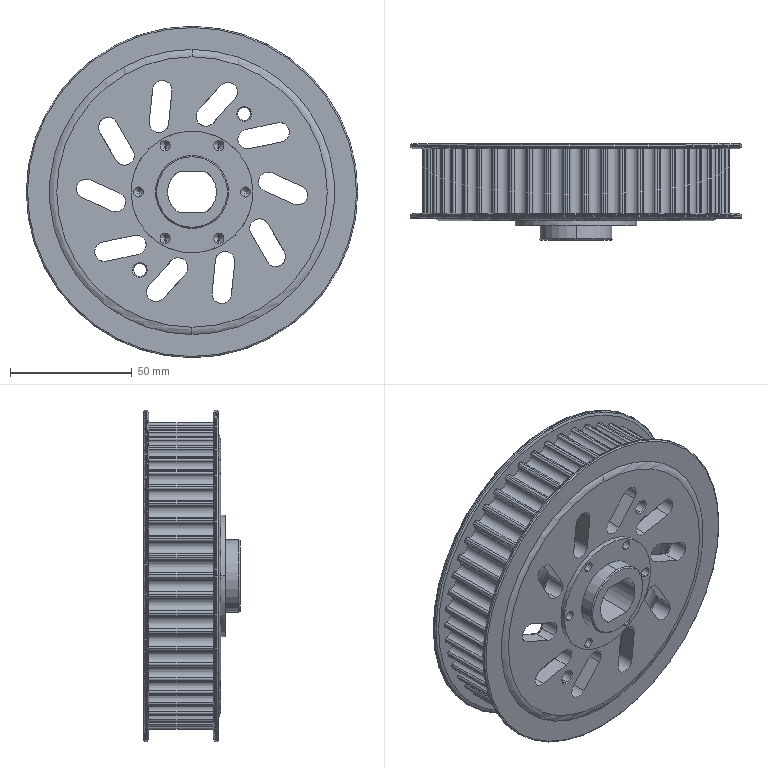Part | SolidWorks | features BaseBody 1 | 1 solid | 428 faces | box 136 x 39.5 x 136 mm | volume 187299 mm3 | cylinder 277 | spline 44 | plane 41 | torus 38 | cone 28 | commonest cylinder face diameters 1.6 x100 5.3 x50 125.95 x50 8 x30 2 x20 4.2 x12